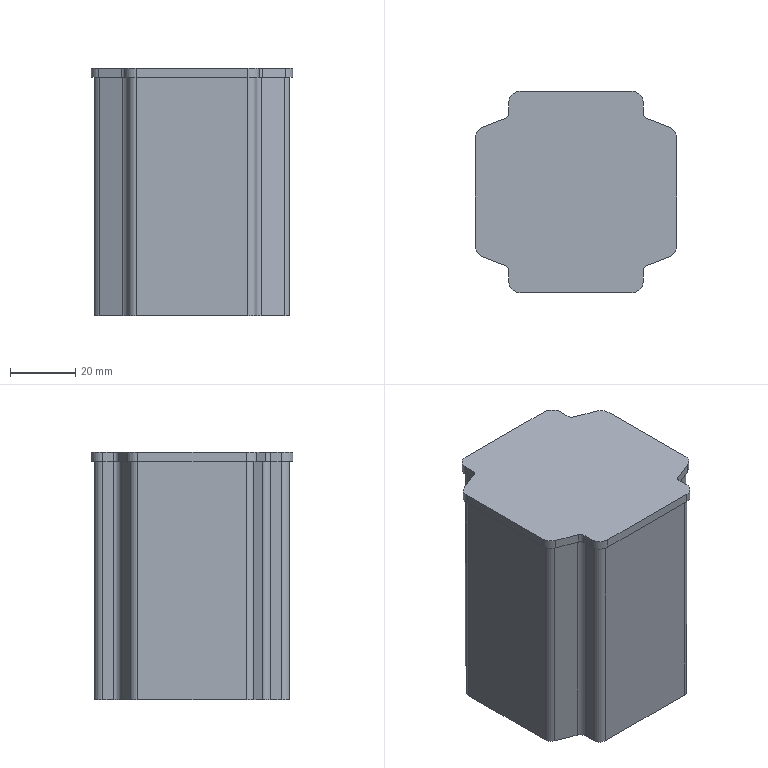Part | STEP file | HF-KE23B_MID | 1 solid | 51 faces | box 62.024 x 62.024 x 76.204 mm | volume 244430 mm3 | plane 27 | cylinder 24 | commonest cylinder face diameters 5.08 x12 7.08 x8 3.08 x4